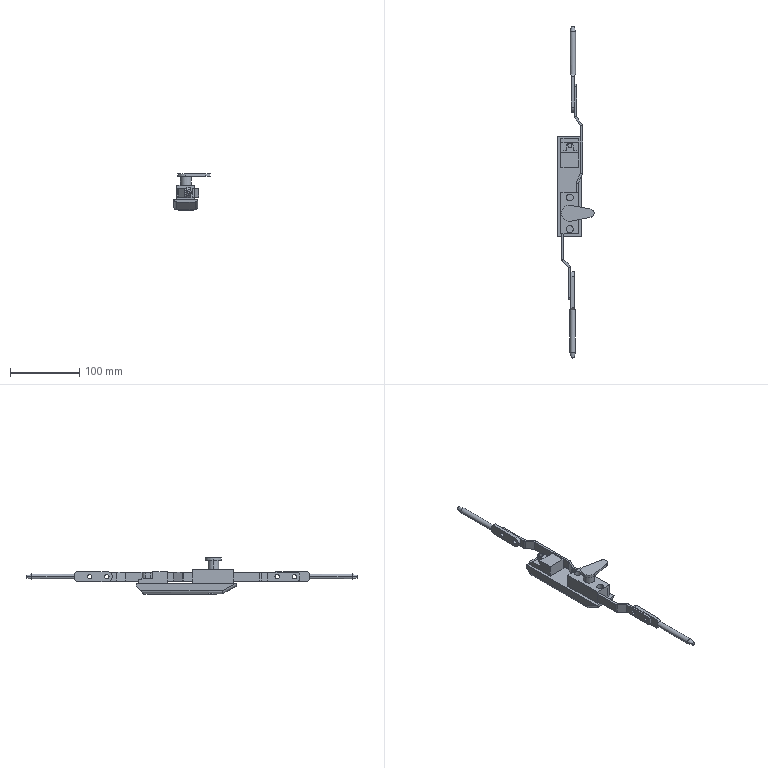Part | SolidWorks | 5 solids | 220 faces | box 52.826 x 480.757 x 53 mm | volume 142243 mm3 | plane 152 | cylinder 64 | cone 4 | commonest cylinder face diameters 6.5 x16 8 x12 1.473 x6 7.473 x6 10 x6 15 x4